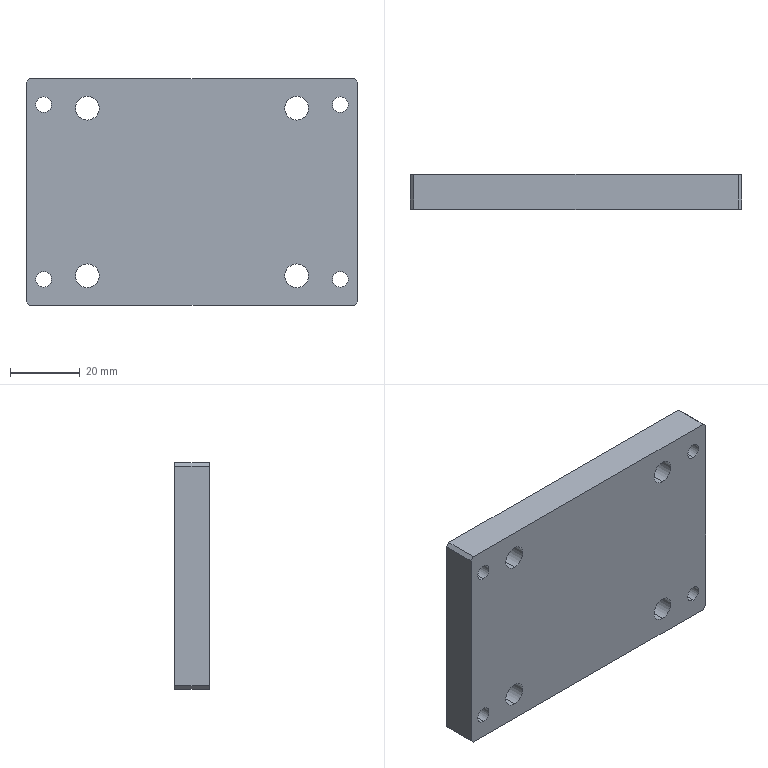Part | SolidWorks | features HoleWzd 2, Chamfer 1, Extrusion 1 | 1 solid | 38 faces | box 95 x 10 x 65 mm | volume 59009 mm3 | cylinder 24 | plane 14 | commonest cylinder face diameters 4.5 x8 6.8 x8 8 x8
STEP:
#1=CARTESIAN_POINT('',(30.,-5.,-27.4));
#2=VERTEX_POINT('',#1);
#3=CARTESIAN_POINT('',(30.,-5.,-20.6));
#4=VERTEX_POINT('',#3);
#5=CARTESIAN_POINT('',(30.,-5.,-24.));
#6=DIRECTION('',(0.,1.,0.));
#7=DIRECTION('',(0.,0.,1.));
#8=AXIS2_PLACEMENT_3D('',#5,#6,#7);
#9=CIRCLE('',#8,3.4);
#10=EDGE_CURVE('',#2,#4,#9,.T.);
#11=ORIENTED_EDGE('',*,*,#10,.F.);
#12=CARTESIAN_POINT('',(30.,5.,-27.4));
#13=VERTEX_POINT('',#12);
#14=CARTESIAN_POINT('',(30.,5.,-27.4));
#15=DIRECTION('',(0.,1.,0.));
#16=VECTOR('',#15,1000.);
#17=LINE('',#14,#16);
#18=EDGE_CURVE('',#2,#13,#17,.T.);
#19=ORIENTED_EDGE('',*,*,#18,.T.);
#20=CARTESIAN_POINT('',(30.,5.,-20.6));
#21=VERTEX_POINT('',#20);
#22=CARTESIAN_POINT('',(30.,5.,-24.));
#23=DIRECTION('',(0.,1.,0.));
#24=DIRECTION('',(0.,0.,1.));
#25=AXIS2_PLACEMENT_3D('',#22,#23,#24);
#26=CIRCLE('',#25,3.4);
#27=EDGE_CURVE('',#13,#21,#26,.T.);
#28=ORIENTED_EDGE('',*,*,#27,.T.);
#29=CARTESIAN_POINT('',(30.,5.,-20.6));
#30=DIRECTION('',(0.,1.,0.));
#31=VECTOR('',#30,1000.);
#32=LINE('',#29,#31);
#33=EDGE_CURVE('',#4,#21,#32,.T.);
#34=ORIENTED_EDGE('',*,*,#33,.F.);
#35=EDGE_LOOP('',(#11,#19,#28,#34));
#36=FACE_OUTER_BOUND('',#35,.T.);
#37=CARTESIAN_POINT('',(30.,5.,-24.));
#38=DIRECTION('',(0.,1.,0.));
#39=DIRECTION('',(0.,0.,1.));
#40=AXIS2_PLACEMENT_3D('',#37,#38,#39);
#41=CYLINDRICAL_SURFACE('',#40,3.4);
#42=ADVANCED_FACE('',(#36),#41,.F.);
#43=CARTESIAN_POINT('',(30.,-5.,20.6));
#44=VERTEX_POINT('',#43);
#45=CARTESIAN_POINT('',(30.,-5.,27.4));
#46=VERTEX_POINT('',#45);
#47=CARTESIAN_POINT('',(30.,-5.,24.));
#48=DIRECTION('',(0.,1.,0.));
#49=DIRECTION('',(0.,0.,1.));
#50=AXIS2_PLACEMENT_3D('',#47,#48,#49);
#51=CIRCLE('',#50,3.4);
#52=EDGE_CURVE('',#44,#46,#51,.T.);
#53=ORIENTED_EDGE('',*,*,#52,.F.);
#54=CARTESIAN_POINT('',(30.,5.,20.6));
#55=VERTEX_POINT('',#54);
#56=CARTESIAN_POINT('',(30.,5.,20.6));
#57=DIRECTION('',(0.,1.,0.));
#58=VECTOR('',#57,1000.);
#59=LINE('',#56,#58);
#60=EDGE_CURVE('',#44,#55,#59,.T.);
#61=ORIENTED_EDGE('',*,*,#60,.T.);
#62=CARTESIAN_POINT('',(30.,5.,27.4));
#63=VERTEX_POINT('',#62);
#64=CARTESIAN_POINT('',(30.,5.,24.));
#65=DIRECTION('',(0.,1.,0.));
#66=DIRECTION('',(0.,0.,1.));
#67=AXIS2_PLACEMENT_3D('',#64,#65,#66);
#68=CIRCLE('',#67,3.4);
#69=EDGE_CURVE('',#55,#63,#68,.T.);
#70=ORIENTED_EDGE('',*,*,#69,.T.);
#71=CARTESIAN_POINT('',(30.,5.,27.4));
#72=DIRECTION('',(0.,1.,0.));
#73=VECTOR('',#72,1000.);
#74=LINE('',#71,#73);
#75=EDGE_CURVE('',#46,#63,#74,.T.);
#76=ORIENTED_EDGE('',*,*,#75,.F.);
#77=EDGE_LOOP('',(#53,#61,#70,#76));
#78=FACE_OUTER_BOUND('',#77,.T.);
#79=CARTESIAN_POINT('',(30.,5.,24.));
#80=DIRECTION('',(0.,1.,0.));
#81=DIRECTION('',(0.,0.,1.));
#82=AXIS2_PLACEMENT_3D('',#79,#80,#81);
#83=CYLINDRICAL_SURFACE('',#82,3.4);
#84=ADVANCED_FACE('',(#78),#83,.F.);
#85=CARTESIAN_POINT('',(-30.,-5.,20.6));
#86=VERTEX_POINT('',#85);
#87=CARTESIAN_POINT('',(-30.,-5.,27.4));
#88=VERTEX_POINT('',#87);
#89=CARTESIAN_POINT('',(-30.,-5.,24.));
#90=DIRECTION('',(0.,1.,0.));
#91=DIRECTION('',(0.,0.,1.));
#92=AXIS2_PLACEMENT_3D('',#89,#90,#91);
#93=CIRCLE('',#92,3.4);
#94=EDGE_CURVE('',#86,#88,#93,.T.);
#95=ORIENTED_EDGE('',*,*,#94,.F.);
#96=CARTESIAN_POINT('',(-30.,5.,20.6));
#97=VERTEX_POINT('',#96);
#98=CARTESIAN_POINT('',(-30.,5.,20.6));
#99=DIRECTION('',(0.,1.,0.));
#100=VECTOR('',#99,1000.);
#101=LINE('',#98,#100);
#102=EDGE_CURVE('',#86,#97,#101,.T.);
#103=ORIENTED_EDGE('',*,*,#102,.T.);
#104=CARTESIAN_POINT('',(-30.,5.,27.4));
#105=VERTEX_POINT('',#104);
#106=CARTESIAN_POINT('',(-30.,5.,24.));
#107=DIRECTION('',(0.,1.,0.));
#108=DIRECTION('',(0.,0.,1.));
#109=AXIS2_PLACEMENT_3D('',#106,#107,#108);
#110=CIRCLE('',#109,3.4);
#111=EDGE_CURVE('',#97,#105,#110,.T.);
#112=ORIENTED_EDGE('',*,*,#111,.T.);
#113=CARTESIAN_POINT('',(-30.,5.,27.4));
#114=DIRECTION('',(0.,1.,0.));
#115=VECTOR('',#114,1000.);
#116=LINE('',#113,#115);
#117=EDGE_CURVE('',#88,#105,#116,.T.);
#118=ORIENTED_EDGE('',*,*,#117,.F.);
#119=EDGE_LOOP('',(#95,#103,#112,#118));
#120=FACE_OUTER_BOUND('',#119,.T.);
#121=CARTESIAN_POINT('',(-30.,5.,24.));
#122=DIRECTION('',(0.,1.,0.));
#123=DIRECTION('',(0.,0.,1.));
#124=AXIS2_PLACEMENT_3D('',#121,#122,#123);
#125=CYLINDRICAL_SURFACE('',#124,3.4);
#126=ADVANCED_FACE('',(#120),#125,.F.);
#127=CARTESIAN_POINT('',(-30.,-5.,-27.4));
#128=VERTEX_POINT('',#127);
#129=CARTESIAN_POINT('',(-30.,-5.,-20.6));
#130=VERTEX_POINT('',#129);
#131=CARTESIAN_POINT('',(-30.,-5.,-24.));
#132=DIRECTION('',(0.,1.,0.));
#133=DIRECTION('',(0.,0.,1.));
#134=AXIS2_PLACEMENT_3D('',#131,#132,#133);
#135=CIRCLE('',#134,3.4);
#136=EDGE_CURVE('',#128,#130,#135,.T.);
#137=ORIENTED_EDGE('',*,*,#136,.F.);
#138=CARTESIAN_POINT('',(-30.,5.,-27.4));
#139=VERTEX_POINT('',#138);
#140=CARTESIAN_POINT('',(-30.,5.,-27.4));
#141=DIRECTION('',(0.,1.,0.));
#142=VECTOR('',#141,1000.);
#143=LINE('',#140,#142);
#144=EDGE_CURVE('',#128,#139,#143,.T.);
#145=ORIENTED_EDGE('',*,*,#144,.T.);
#146=CARTESIAN_POINT('',(-30.,5.,-20.6));
#147=VERTEX_POINT('',#146);
#148=CARTESIAN_POINT('',(-30.,5.,-24.));
#149=DIRECTION('',(0.,1.,0.));
#150=DIRECTION('',(0.,0.,1.));
#151=AXIS2_PLACEMENT_3D('',#148,#149,#150);
#152=CIRCLE('',#151,3.4);
#153=EDGE_CURVE('',#139,#147,#152,.T.);
#154=ORIENTED_EDGE('',*,*,#153,.T.);
#155=CARTESIAN_POINT('',(-30.,5.,-20.6));
#156=DIRECTION('',(0.,1.,0.));
#157=VECTOR('',#156,1000.);
#158=LINE('',#155,#157);
#159=EDGE_CURVE('',#130,#147,#158,.T.);
#160=ORIENTED_EDGE('',*,*,#159,.F.);
#161=EDGE_LOOP('',(#137,#145,#154,#160));
#162=FACE_OUTER_BOUND('',#161,.T.);
#163=CARTESIAN_POINT('',(-30.,5.,-24.));
#164=DIRECTION('',(0.,1.,0.));
#165=DIRECTION('',(0.,0.,1.));
#166=AXIS2_PLACEMENT_3D('',#163,#164,#165);
#167=CYLINDRICAL_SURFACE('',#166,3.4);
#168=ADVANCED_FACE('',(#162),#167,.F.);
#169=CARTESIAN_POINT('',(-42.5,0.4,-29.));
#170=VERTEX_POINT('',#169);
#171=CARTESIAN_POINT('',(-42.5,0.4,-21.));
#172=VERTEX_POINT('',#171);
#173=CARTESIAN_POINT('',(-42.5,0.4,-25.));
#174=DIRECTION('',(0.,1.,0.));
#175=DIRECTION('',(0.,0.,1.));
#176=AXIS2_PLACEMENT_3D('',#173,#174,#175);
#177=CIRCLE('',#176,4.);
#178=EDGE_CURVE('',#170,#172,#177,.T.);
#179=ORIENTED_EDGE('',*,*,#178,.F.);
#180=CARTESIAN_POINT('',(-42.5,5.,-29.));
#181=VERTEX_POINT('',#180);
#182=CARTESIAN_POINT('',(-42.5,5.,-29.));
#183=DIRECTION('',(0.,1.,0.));
#184=VECTOR('',#183,1000.);
#185=LINE('',#182,#184);
#186=EDGE_CURVE('',#170,#181,#185,.T.);
#187=ORIENTED_EDGE('',*,*,#186,.T.);
#188=CARTESIAN_POINT('',(-42.5,5.,-21.));
#189=VERTEX_POINT('',#188);
#190=CARTESIAN_POINT('',(-42.5,5.,-25.));
#191=DIRECTION('',(0.,1.,0.));
#192=DIRECTION('',(0.,0.,1.));
#193=AXIS2_PLACEMENT_3D('',#190,#191,#192);
#194=CIRCLE('',#193,4.);
#195=EDGE_CURVE('',#181,#189,#194,.T.);
#196=ORIENTED_EDGE('',*,*,#195,.T.);
#197=CARTESIAN_POINT('',(-42.5,5.,-21.));
#198=DIRECTION('',(0.,1.,0.));
#199=VECTOR('',#198,1000.);
#200=LINE('',#197,#199);
#201=EDGE_CURVE('',#172,#189,#200,.T.);
#202=ORIENTED_EDGE('',*,*,#201,.F.);
#203=EDGE_LOOP('',(#179,#187,#196,#202));
#204=FACE_OUTER_BOUND('',#203,.T.);
#205=CARTESIAN_POINT('',(-42.5,5.,-25.));
#206=DIRECTION('',(0.,1.,0.));
#207=DIRECTION('',(0.,0.,1.));
#208=AXIS2_PLACEMENT_3D('',#205,#206,#207);
#209=CYLINDRICAL_SURFACE('',#208,4.);
#210=ADVANCED_FACE('',(#204),#209,.F.);
#211=CARTESIAN_POINT('',(-42.5,-5.,-27.25));
#212=VERTEX_POINT('',#211);
#213=CARTESIAN_POINT('',(-42.5,-5.,-22.75));
#214=VERTEX_POINT('',#213);
#215=CARTESIAN_POINT('',(-42.5,-5.,-25.));
#216=DIRECTION('',(0.,1.,0.));
#217=DIRECTION('',(0.,0.,1.));
#218=AXIS2_PLACEMENT_3D('',#215,#216,#217);
#219=CIRCLE('',#218,2.25);
#220=EDGE_CURVE('',#212,#214,#219,.T.);
#221=ORIENTED_EDGE('',*,*,#220,.F.);
#222=CARTESIAN_POINT('',(-42.5,0.4,-27.25));
#223=VERTEX_POINT('',#222);
#224=CARTESIAN_POINT('',(-42.5,5.,-27.25));
#225=DIRECTION('',(0.,1.,0.));
#226=VECTOR('',#225,1000.);
#227=LINE('',#224,#226);
#228=EDGE_CURVE('',#212,#223,#227,.T.);
#229=ORIENTED_EDGE('',*,*,#228,.T.);
#230=CARTESIAN_POINT('',(-42.5,0.4,-22.75));
#231=VERTEX_POINT('',#230);
#232=CARTESIAN_POINT('',(-42.5,0.4,-25.));
#233=DIRECTION('',(0.,1.,0.));
#234=DIRECTION('',(0.,0.,1.));
#235=AXIS2_PLACEMENT_3D('',#232,#233,#234);
#236=CIRCLE('',#235,2.25);
#237=EDGE_CURVE('',#223,#231,#236,.T.);
#238=ORIENTED_EDGE('',*,*,#237,.T.);
#239=CARTESIAN_POINT('',(-42.5,5.,-22.75));
#240=DIRECTION('',(0.,1.,0.));
#241=VECTOR('',#240,1000.);
#242=LINE('',#239,#241);
#243=EDGE_CURVE('',#214,#231,#242,.T.);
#244=ORIENTED_EDGE('',*,*,#243,.F.);
#245=EDGE_LOOP('',(#221,#229,#238,#244));
#246=FACE_OUTER_BOUND('',#245,.T.);
#247=CARTESIAN_POINT('',(-42.5,5.,-25.));
#248=DIRECTION('',(0.,1.,0.));
#249=DIRECTION('',(0.,0.,1.));
#250=AXIS2_PLACEMENT_3D('',#247,#248,#249);
#251=CYLINDRICAL_SURFACE('',#250,2.25);
#252=ADVANCED_FACE('',(#246),#251,.F.);
#253=CARTESIAN_POINT('',(-42.5,0.4,21.));
#254=VERTEX_POINT('',#253);
#255=CARTESIAN_POINT('',(-42.5,0.4,29.));
#256=VERTEX_POINT('',#255);
#257=CARTESIAN_POINT('',(-42.5,0.4,25.));
#258=DIRECTION('',(0.,1.,0.));
#259=DIRECTION('',(0.,0.,1.));
#260=AXIS2_PLACEMENT_3D('',#257,#258,#259);
#261=CIRCLE('',#260,4.);
#262=EDGE_CURVE('',#254,#256,#261,.T.);
#263=ORIENTED_EDGE('',*,*,#262,.F.);
#264=CARTESIAN_POINT('',(-42.5,5.,21.));
#265=VERTEX_POINT('',#264);
#266=CARTESIAN_POINT('',(-42.5,5.,21.));
#267=DIRECTION('',(0.,1.,0.));
#268=VECTOR('',#267,1000.);
#269=LINE('',#266,#268);
#270=EDGE_CURVE('',#254,#265,#269,.T.);
#271=ORIENTED_EDGE('',*,*,#270,.T.);
#272=CARTESIAN_POINT('',(-42.5,5.,29.));
#273=VERTEX_POINT('',#272);
#274=CARTESIAN_POINT('',(-42.5,5.,25.));
#275=DIRECTION('',(0.,1.,0.));
#276=DIRECTION('',(0.,0.,1.));
#277=AXIS2_PLACEMENT_3D('',#274,#275,#276);
#278=CIRCLE('',#277,4.);
#279=EDGE_CURVE('',#265,#273,#278,.T.);
#280=ORIENTED_EDGE('',*,*,#279,.T.);
#281=CARTESIAN_POINT('',(-42.5,5.,29.));
#282=DIRECTION('',(0.,1.,0.));
#283=VECTOR('',#282,1000.);
#284=LINE('',#281,#283);
#285=EDGE_CURVE('',#256,#273,#284,.T.);
#286=ORIENTED_EDGE('',*,*,#285,.F.);
#287=EDGE_LOOP('',(#263,#271,#280,#286));
#288=FACE_OUTER_BOUND('',#287,.T.);
#289=CARTESIAN_POINT('',(-42.5,5.,25.));
#290=DIRECTION('',(0.,1.,0.));
#291=DIRECTION('',(0.,0.,1.));
#292=AXIS2_PLACEMENT_3D('',#289,#290,#291);
#293=CYLINDRICAL_SURFACE('',#292,4.);
#294=ADVANCED_FACE('',(#288),#293,.F.);
#295=CARTESIAN_POINT('',(-42.5,-5.,22.75));
#296=VERTEX_POINT('',#295);
#297=CARTESIAN_POINT('',(-42.5,-5.,27.25));
#298=VERTEX_POINT('',#297);
#299=CARTESIAN_POINT('',(-42.5,-5.,25.));
#300=DIRECTION('',(0.,1.,0.));
#301=DIRECTION('',(0.,0.,1.));
#302=AXIS2_PLACEMENT_3D('',#299,#300,#301);
#303=CIRCLE('',#302,2.25);
#304=EDGE_CURVE('',#296,#298,#303,.T.);
#305=ORIENTED_EDGE('',*,*,#304,.F.);
#306=CARTESIAN_POINT('',(-42.5,0.4,22.75));
#307=VERTEX_POINT('',#306);
#308=CARTESIAN_POINT('',(-42.5,5.,22.75));
#309=DIRECTION('',(0.,1.,0.));
#310=VECTOR('',#309,1000.);
#311=LINE('',#308,#310);
#312=EDGE_CURVE('',#296,#307,#311,.T.);
#313=ORIENTED_EDGE('',*,*,#312,.T.);
#314=CARTESIAN_POINT('',(-42.5,0.4,27.25));
#315=VERTEX_POINT('',#314);
#316=CARTESIAN_POINT('',(-42.5,0.4,25.));
#317=DIRECTION('',(0.,1.,0.));
#318=DIRECTION('',(0.,0.,1.));
#319=AXIS2_PLACEMENT_3D('',#316,#317,#318);
#320=CIRCLE('',#319,2.25);
#321=EDGE_CURVE('',#307,#315,#320,.T.);
#322=ORIENTED_EDGE('',*,*,#321,.T.);
#323=CARTESIAN_POINT('',(-42.5,5.,27.25));
#324=DIRECTION('',(0.,1.,0.));
#325=VECTOR('',#324,1000.);
#326=LINE('',#323,#325);
#327=EDGE_CURVE('',#298,#315,#326,.T.);
#328=ORIENTED_EDGE('',*,*,#327,.F.);
#329=EDGE_LOOP('',(#305,#313,#322,#328));
#330=FACE_OUTER_BOUND('',#329,.T.);
#331=CARTESIAN_POINT('',(-42.5,5.,25.));
#332=DIRECTION('',(0.,1.,0.));
#333=DIRECTION('',(0.,0.,1.));
#334=AXIS2_PLACEMENT_3D('',#331,#332,#333);
#335=CYLINDRICAL_SURFACE('',#334,2.25);
#336=ADVANCED_FACE('',(#330),#335,.F.);
#337=CARTESIAN_POINT('',(42.5,0.4,21.));
#338=VERTEX_POINT('',#337);
#339=CARTESIAN_POINT('',(42.5,0.4,29.));
#340=VERTEX_POINT('',#339);
#341=CARTESIAN_POINT('',(42.5,0.4,25.));
#342=DIRECTION('',(0.,1.,0.));
#343=DIRECTION('',(0.,0.,1.));
#344=AXIS2_PLACEMENT_3D('',#341,#342,#343);
#345=CIRCLE('',#344,4.);
#346=EDGE_CURVE('',#338,#340,#345,.T.);
#347=ORIENTED_EDGE('',*,*,#346,.F.);
#348=CARTESIAN_POINT('',(42.5,5.,21.));
#349=VERTEX_POINT('',#348);
#350=CARTESIAN_POINT('',(42.5,5.,21.));
#351=DIRECTION('',(0.,1.,0.));
#352=VECTOR('',#351,1000.);
#353=LINE('',#350,#352);
#354=EDGE_CURVE('',#338,#349,#353,.T.);
#355=ORIENTED_EDGE('',*,*,#354,.T.);
#356=CARTESIAN_POINT('',(42.5,5.,29.));
#357=VERTEX_POINT('',#356);
#358=CARTESIAN_POINT('',(42.5,5.,25.));
#359=DIRECTION('',(0.,1.,0.));
#360=DIRECTION('',(0.,0.,1.));
#361=AXIS2_PLACEMENT_3D('',#358,#359,#360);
#362=CIRCLE('',#361,4.);
#363=EDGE_CURVE('',#349,#357,#362,.T.);
#364=ORIENTED_EDGE('',*,*,#363,.T.);
#365=CARTESIAN_POINT('',(42.5,5.,29.));
#366=DIRECTION('',(0.,1.,0.));
#367=VECTOR('',#366,1000.);
#368=LINE('',#365,#367);
#369=EDGE_CURVE('',#340,#357,#368,.T.);
#370=ORIENTED_EDGE('',*,*,#369,.F.);
#371=EDGE_LOOP('',(#347,#355,#364,#370));
#372=FACE_OUTER_BOUND('',#371,.T.);
#373=CARTESIAN_POINT('',(42.5,5.,25.));
#374=DIRECTION('',(0.,1.,0.));
#375=DIRECTION('',(0.,0.,1.));
#376=AXIS2_PLACEMENT_3D('',#373,#374,#375);
#377=CYLINDRICAL_SURFACE('',#376,4.);
#378=ADVANCED_FACE('',(#372),#377,.F.);
#379=CARTESIAN_POINT('',(42.5,-5.,22.75));
#380=VERTEX_POINT('',#379);
#381=CARTESIAN_POINT('',(42.5,-5.,27.25));
#382=VERTEX_POINT('',#381);
#383=CARTESIAN_POINT('',(42.5,-5.,25.));
#384=DIRECTION('',(0.,1.,0.));
#385=DIRECTION('',(0.,0.,1.));
#386=AXIS2_PLACEMENT_3D('',#383,#384,#385);
#387=CIRCLE('',#386,2.25);
#388=EDGE_CURVE('',#380,#382,#387,.T.);
#389=ORIENTED_EDGE('',*,*,#388,.F.);
#390=CARTESIAN_POINT('',(42.5,0.4,22.75));
#391=VERTEX_POINT('',#390);
#392=CARTESIAN_POINT('',(42.5,5.,22.75));
#393=DIRECTION('',(0.,1.,0.));
#394=VECTOR('',#393,1000.);
#395=LINE('',#392,#394);
#396=EDGE_CURVE('',#380,#391,#395,.T.);
#397=ORIENTED_EDGE('',*,*,#396,.T.);
#398=CARTESIAN_POINT('',(42.5,0.4,27.25));
#399=VERTEX_POINT('',#398);
#400=CARTESIAN_POINT('',(42.5,0.4,25.));
#401=DIRECTION('',(0.,1.,0.));
#402=DIRECTION('',(0.,0.,1.));
#403=AXIS2_PLACEMENT_3D('',#400,#401,#402);
#404=CIRCLE('',#403,2.25);
#405=EDGE_CURVE('',#391,#399,#404,.T.);
#406=ORIENTED_EDGE('',*,*,#405,.T.);
#407=CARTESIAN_POINT('',(42.5,5.,27.25));
#408=DIRECTION('',(0.,1.,0.));
#409=VECTOR('',#408,1000.);
#410=LINE('',#407,#409);
#411=EDGE_CURVE('',#382,#399,#410,.T.);
#412=ORIENTED_EDGE('',*,*,#411,.F.);
#413=EDGE_LOOP('',(#389,#397,#406,#412));
#414=FACE_OUTER_BOUND('',#413,.T.);
#415=CARTESIAN_POINT('',(42.5,5.,25.));
#416=DIRECTION('',(0.,1.,0.));
#417=DIRECTION('',(0.,0.,1.));
#418=AXIS2_PLACEMENT_3D('',#415,#416,#417);
#419=CYLINDRICAL_SURFACE('',#418,2.25);
#420=ADVANCED_FACE('',(#414),#419,.F.);
#421=CARTESIAN_POINT('',(42.5,0.4,-29.));
#422=VERTEX_POINT('',#421);
#423=CARTESIAN_POINT('',(42.5,0.4,-21.));
#424=VERTEX_POINT('',#423);
#425=CARTESIAN_POINT('',(42.5,0.4,-25.));
#426=DIRECTION('',(0.,1.,0.));
#427=DIRECTION('',(0.,0.,1.));
#428=AXIS2_PLACEMENT_3D('',#425,#426,#427);
#429=CIRCLE('',#428,4.);
#430=EDGE_CURVE('',#422,#424,#429,.T.);
#431=ORIENTED_EDGE('',*,*,#430,.F.);
#432=CARTESIAN_POINT('',(42.5,5.,-29.));
#433=VERTEX_POINT('',#432);
#434=CARTESIAN_POINT('',(42.5,5.,-29.));
#435=DIRECTION('',(0.,1.,0.));
#436=VECTOR('',#435,1000.);
#437=LINE('',#434,#436);
#438=EDGE_CURVE('',#422,#433,#437,.T.);
#439=ORIENTED_EDGE('',*,*,#438,.T.);
#440=CARTESIAN_POINT('',(42.5,5.,-21.));
#441=VERTEX_POINT('',#440);
#442=CARTESIAN_POINT('',(42.5,5.,-25.));
#443=DIRECTION('',(0.,1.,0.));
#444=DIRECTION('',(0.,0.,1.));
#445=AXIS2_PLACEMENT_3D('',#442,#443,#444);
#446=CIRCLE('',#445,4.);
#447=EDGE_CURVE('',#433,#441,#446,.T.);
#448=ORIENTED_EDGE('',*,*,#447,.T.);
#449=CARTESIAN_POINT('',(42.5,5.,-21.));
#450=DIRECTION('',(0.,1.,0.));
#451=VECTOR('',#450,1000.);
#452=LINE('',#449,#451);
#453=EDGE_CURVE('',#424,#441,#452,.T.);
#454=ORIENTED_EDGE('',*,*,#453,.F.);
#455=EDGE_LOOP('',(#431,#439,#448,#454));
#456=FACE_OUTER_BOUND('',#455,.T.);
#457=CARTESIAN_POINT('',(42.5,5.,-25.));
#458=DIRECTION('',(0.,1.,0.));
#459=DIRECTION('',(0.,0.,1.));
#460=AXIS2_PLACEMENT_3D('',#457,#458,#459);
#461=CYLINDRICAL_SURFACE('',#460,4.);
#462=ADVANCED_FACE('',(#456),#461,.F.);
#463=CARTESIAN_POINT('',(42.5,-5.,-27.25));
#464=VERTEX_POINT('',#463);
#465=CARTESIAN_POINT('',(42.5,-5.,-22.75));
#466=VERTEX_POINT('',#465);
#467=CARTESIAN_POINT('',(42.5,-5.,-25.));
#468=DIRECTION('',(0.,1.,0.));
#469=DIRECTION('',(0.,0.,1.));
#470=AXIS2_PLACEMENT_3D('',#467,#468,#469);
#471=CIRCLE('',#470,2.25);
#472=EDGE_CURVE('',#464,#466,#471,.T.);
#473=ORIENTED_EDGE('',*,*,#472,.F.);
#474=CARTESIAN_POINT('',(42.5,0.4,-27.25));
#475=VERTEX_POINT('',#474);
#476=CARTESIAN_POINT('',(42.5,5.,-27.25));
#477=DIRECTION('',(0.,1.,0.));
#478=VECTOR('',#477,1000.);
#479=LINE('',#476,#478);
#480=EDGE_CURVE('',#464,#475,#479,.T.);
#481=ORIENTED_EDGE('',*,*,#480,.T.);
#482=CARTESIAN_POINT('',(42.5,0.4,-22.75));
#483=VERTEX_POINT('',#482);
#484=CARTESIAN_POINT('',(42.5,0.4,-25.));
#485=DIRECTION('',(0.,1.,0.));
#486=DIRECTION('',(0.,0.,1.));
#487=AXIS2_PLACEMENT_3D('',#484,#485,#486);
#488=CIRCLE('',#487,2.25);
#489=EDGE_CURVE('',#475,#483,#488,.T.);
#490=ORIENTED_EDGE('',*,*,#489,.T.);
#491=CARTESIAN_POINT('',(42.5,5.,-22.75));
#492=DIRECTION('',(0.,1.,0.));
#493=VECTOR('',#492,1000.);
#494=LINE('',#491,#493);
#495=EDGE_CURVE('',#466,#483,#494,.T.);
#496=ORIENTED_EDGE('',*,*,#495,.F.);
#497=EDGE_LOOP('',(#473,#481,#490,#496));
#498=FACE_OUTER_BOUND('',#497,.T.);
#499=CARTESIAN_POINT('',(42.5,5.,-25.));
#500=DIRECTION('',(0.,1.,0.));
#501=DIRECTION('',(0.,0.,1.));
#502=AXIS2_PLACEMENT_3D('',#499,#500,#501);
#503=CYLINDRICAL_SURFACE('',#502,2.25);
#504=ADVANCED_FACE('',(#498),#503,.F.);
#505=CARTESIAN_POINT('',(30.,-5.,-24.));
#506=DIRECTION('',(0.,1.,0.));
#507=DIRECTION('',(0.,0.,1.));
#508=AXIS2_PLACEMENT_3D('',#505,#506,#507);
#509=CIRCLE('',#508,3.4);
#510=EDGE_CURVE('',#4,#2,#509,.T.);
#511=ORIENTED_EDGE('',*,*,#510,.T.);
#512=ORIENTED_EDGE('',*,*,#10,.T.);
#513=EDGE_LOOP('',(#511,#512));
#514=FACE_BOUND('',#513,.T.);
#515=CARTESIAN_POINT('',(30.,-5.,24.));
#516=DIRECTION('',(0.,1.,0.));
#517=DIRECTION('',(0.,0.,1.));
#518=AXIS2_PLACEMENT_3D('',#515,#516,#517);
#519=CIRCLE('',#518,3.4);
#520=EDGE_CURVE('',#46,#44,#519,.T.);
#521=ORIENTED_EDGE('',*,*,#520,.T.);
#522=ORIENTED_EDGE('',*,*,#52,.T.);
#523=EDGE_LOOP('',(#521,#522));
#524=FACE_BOUND('',#523,.T.);
#525=CARTESIAN_POINT('',(-30.,-5.,24.));
#526=DIRECTION('',(0.,1.,0.));
#527=DIRECTION('',(0.,0.,1.));
#528=AXIS2_PLACEMENT_3D('',#525,#526,#527);
#529=CIRCLE('',#528,3.4);
#530=EDGE_CURVE('',#88,#86,#529,.T.);
#531=ORIENTED_EDGE('',*,*,#530,.T.);
#532=ORIENTED_EDGE('',*,*,#94,.T.);
#533=EDGE_LOOP('',(#531,#532));
#534=FACE_BOUND('',#533,.T.);
#535=CARTESIAN_POINT('',(46.5,-5.,-32.5));
#536=VERTEX_POINT('',#535);
#537=CARTESIAN_POINT('',(-46.5,-5.,-32.5));
#538=VERTEX_POINT('',#537);
#539=CARTESIAN_POINT('',(-47.5,-5.,-32.5));
#540=DIRECTION('',(-1.,0.,0.));
#541=VECTOR('',#540,1000.);
#542=LINE('',#539,#541);
#543=EDGE_CURVE('',#536,#538,#542,.T.);
#544=ORIENTED_EDGE('',*,*,#543,.F.);
#545=CARTESIAN_POINT('',(47.5,-5.,-31.5));
#546=VERTEX_POINT('',#545);
#547=CARTESIAN_POINT('',(39.5,-5.,-39.5));
#548=DIRECTION('',(0.7071,0.,0.7071));
#549=VECTOR('',#548,1000.);
#550=LINE('',#547,#549);
#551=EDGE_CURVE('',#536,#546,#550,.T.);
#552=ORIENTED_EDGE('',*,*,#551,.T.);
#553=CARTESIAN_POINT('',(47.5,-5.,31.5));
#554=VERTEX_POINT('',#553);
#555=CARTESIAN_POINT('',(47.5,-5.,32.5));
#556=DIRECTION('',(0.,0.,-1.));
#557=VECTOR('',#556,1000.);
#558=LINE('',#555,#557);
#559=EDGE_CURVE('',#554,#546,#558,.T.);
#560=ORIENTED_EDGE('',*,*,#559,.F.);
#561=CARTESIAN_POINT('',(46.5,-5.,32.5));
#562=VERTEX_POINT('',#561);
#563=CARTESIAN_POINT('',(39.5,-5.,39.5));
#564=DIRECTION('',(-0.7071,0.,0.7071));
#565=VECTOR('',#564,1000.);
#566=LINE('',#563,#565);
#567=EDGE_CURVE('',#554,#562,#566,.T.);
#568=ORIENTED_EDGE('',*,*,#567,.T.);
#569=CARTESIAN_POINT('',(-46.5,-5.,32.5));
#570=VERTEX_POINT('',#569);
#571=CARTESIAN_POINT('',(-47.5,-5.,32.5));
#572=DIRECTION('',(1.,0.,0.));
#573=VECTOR('',#572,1000.);
#574=LINE('',#571,#573);
#575=EDGE_CURVE('',#570,#562,#574,.T.);
#576=ORIENTED_EDGE('',*,*,#575,.F.);
#577=CARTESIAN_POINT('',(-47.5,-5.,31.5));
#578=VERTEX_POINT('',#577);
#579=CARTESIAN_POINT('',(-39.5,-5.,39.5));
#580=DIRECTION('',(-0.7071,0.,-0.7071));
#581=VECTOR('',#580,1000.);
#582=LINE('',#579,#581);
#583=EDGE_CURVE('',#570,#578,#582,.T.);
#584=ORIENTED_EDGE('',*,*,#583,.T.);
#585=CARTESIAN_POINT('',(-47.5,-5.,-31.5));
#586=VERTEX_POINT('',#585);
#587=CARTESIAN_POINT('',(-47.5,-5.,32.5));
#588=DIRECTION('',(0.,0.,1.));
#589=VECTOR('',#588,1000.);
#590=LINE('',#587,#589);
#591=EDGE_CURVE('',#586,#578,#590,.T.);
#592=ORIENTED_EDGE('',*,*,#591,.F.);
#593=CARTESIAN_POINT('',(-39.5,-5.,-39.5));
#594=DIRECTION('',(0.7071,0.,-0.7071));
#595=VECTOR('',#594,1000.);
#596=LINE('',#593,#595);
#597=EDGE_CURVE('',#586,#538,#596,.T.);
#598=ORIENTED_EDGE('',*,*,#597,.T.);
#599=EDGE_LOOP('',(#544,#552,#560,#568,#576,#584,#592,#598));
#600=FACE_OUTER_BOUND('',#599,.T.);
#601=CARTESIAN_POINT('',(42.5,-5.,-25.));
#602=DIRECTION('',(0.,1.,0.));
#603=DIRECTION('',(0.,0.,1.));
#604=AXIS2_PLACEMENT_3D('',#601,#602,#603);
#605=CIRCLE('',#604,2.25);
#606=EDGE_CURVE('',#466,#464,#605,.T.);
#607=ORIENTED_EDGE('',*,*,#606,.T.);
#608=ORIENTED_EDGE('',*,*,#472,.T.);
#609=EDGE_LOOP('',(#607,#608));
#610=FACE_BOUND('',#609,.T.);
#611=CARTESIAN_POINT('',(42.5,-5.,25.));
#612=DIRECTION('',(0.,1.,0.));
#613=DIRECTION('',(0.,0.,1.));
#614=AXIS2_PLACEMENT_3D('',#611,#612,#613);
#615=CIRCLE('',#614,2.25);
#616=EDGE_CURVE('',#382,#380,#615,.T.);
#617=ORIENTED_EDGE('',*,*,#616,.T.);
#618=ORIENTED_EDGE('',*,*,#388,.T.);
#619=EDGE_LOOP('',(#617,#618));
#620=FACE_BOUND('',#619,.T.);
#621=CARTESIAN_POINT('',(-42.5,-5.,25.));
#622=DIRECTION('',(0.,1.,0.));
#623=DIRECTION('',(0.,0.,1.));
#624=AXIS2_PLACEMENT_3D('',#621,#622,#623);
#625=CIRCLE('',#624,2.25);
#626=EDGE_CURVE('',#298,#296,#625,.T.);
#627=ORIENTED_EDGE('',*,*,#626,.T.);
#628=ORIENTED_EDGE('',*,*,#304,.T.);
#629=EDGE_LOOP('',(#627,#628));
#630=FACE_BOUND('',#629,.T.);
#631=CARTESIAN_POINT('',(-42.5,-5.,-25.));
#632=DIRECTION('',(0.,1.,0.));
#633=DIRECTION('',(0.,0.,1.));
#634=AXIS2_PLACEMENT_3D('',#631,#632,#633);
#635=CIRCLE('',#634,2.25);
#636=EDGE_CURVE('',#214,#212,#635,.T.);
#637=ORIENTED_EDGE('',*,*,#636,.T.);
#638=ORIENTED_EDGE('',*,*,#220,.T.);
#639=EDGE_LOOP('',(#637,#638));
#640=FACE_BOUND('',#639,.T.);
#641=CARTESIAN_POINT('',(-30.,-5.,-24.));
#642=DIRECTION('',(0.,1.,0.));
#643=DIRECTION('',(0.,0.,1.));
#644=AXIS2_PLACEMENT_3D('',#641,#642,#643);
#645=CIRCLE('',#644,3.4);
#646=EDGE_CURVE('',#130,#128,#645,.T.);
#647=ORIENTED_EDGE('',*,*,#646,.T.);
#648=ORIENTED_EDGE('',*,*,#136,.T.);
#649=EDGE_LOOP('',(#647,#648));
#650=FACE_BOUND('',#649,.T.);
#651=CARTESIAN_POINT('',(0.,-5.,0.));
#652=DIRECTION('',(0.,-1.,0.));
#653=DIRECTION('',(0.,0.,-1.));
#654=AXIS2_PLACEMENT_3D('',#651,#652,#653);
#655=PLANE('',#654);
#656=ADVANCED_FACE('',(#514,#524,#534,#600,#610,#620,#630,#640,#650),#655,.T.);
#657=ORIENTED_EDGE('',*,*,#559,.T.);
#658=CARTESIAN_POINT('',(47.5,5.,-31.5));
#659=VERTEX_POINT('',#658);
#660=CARTESIAN_POINT('',(47.5,5.,-31.5));
#661=DIRECTION('',(0.,1.,0.));
#662=VECTOR('',#661,1000.);
#663=LINE('',#660,#662);
#664=EDGE_CURVE('',#546,#659,#663,.T.);
#665=ORIENTED_EDGE('',*,*,#664,.T.);
#666=CARTESIAN_POINT('',(47.5,5.,31.5));
#667=VERTEX_POINT('',#666);
#668=CARTESIAN_POINT('',(47.5,5.,32.5));
#669=DIRECTION('',(0.,0.,-1.));
#670=VECTOR('',#669,1000.);
#671=LINE('',#668,#670);
#672=EDGE_CURVE('',#667,#659,#671,.T.);
#673=ORIENTED_EDGE('',*,*,#672,.F.);
#674=CARTESIAN_POINT('',(47.5,5.,31.5));
#675=DIRECTION('',(0.,-1.,0.));
#676=VECTOR('',#675,1000.);
#677=LINE('',#674,#676);
#678=EDGE_CURVE('',#667,#554,#677,.T.);
#679=ORIENTED_EDGE('',*,*,#678,.T.);
#680=EDGE_LOOP('',(#657,#665,#673,#679));
#681=FACE_OUTER_BOUND('',#680,.T.);
#682=CARTESIAN_POINT('',(47.5,5.,32.5));
#683=DIRECTION('',(-1.,0.,0.));
#684=DIRECTION('',(0.,0.,1.));
#685=AXIS2_PLACEMENT_3D('',#682,#683,#684);
#686=PLANE('',#685);
#687=ADVANCED_FACE('',(#681),#686,.F.);
#688=CARTESIAN_POINT('',(46.5,5.,-32.5));
#689=VERTEX_POINT('',#688);
#690=CARTESIAN_POINT('',(-46.5,5.,-32.5));
#691=VERTEX_POINT('',#690);
#692=CARTESIAN_POINT('',(-47.5,5.,-32.5));
#693=DIRECTION('',(-1.,0.,0.));
#694=VECTOR('',#693,1000.);
#695=LINE('',#692,#694);
#696=EDGE_CURVE('',#689,#691,#695,.T.);
#697=ORIENTED_EDGE('',*,*,#696,.F.);
#698=CARTESIAN_POINT('',(46.5,5.,-32.5));
#699=DIRECTION('',(0.,-1.,0.));
#700=VECTOR('',#699,1000.);
#701=LINE('',#698,#700);
#702=EDGE_CURVE('',#689,#536,#701,.T.);
#703=ORIENTED_EDGE('',*,*,#702,.T.);
#704=ORIENTED_EDGE('',*,*,#543,.T.);
#705=CARTESIAN_POINT('',(-46.5,5.,-32.5));
#706=DIRECTION('',(0.,1.,0.));
#707=VECTOR('',#706,1000.);
#708=LINE('',#705,#707);
#709=EDGE_CURVE('',#538,#691,#708,.T.);
#710=ORIENTED_EDGE('',*,*,#709,.T.);
#711=EDGE_LOOP('',(#697,#703,#704,#710));
#712=FACE_OUTER_BOUND('',#711,.T.);
#713=CARTESIAN_POINT('',(-47.5,5.,-32.5));
#714=DIRECTION('',(0.,0.,1.));
#715=DIRECTION('',(1.,0.,0.));
#716=AXIS2_PLACEMENT_3D('',#713,#714,#715);
#717=PLANE('',#716);
#718=ADVANCED_FACE('',(#712),#717,.F.);
#719=ORIENTED_EDGE('',*,*,#591,.T.);
#720=CARTESIAN_POINT('',(-47.5,5.,31.5));
#721=VERTEX_POINT('',#720);
#722=CARTESIAN_POINT('',(-47.5,5.,31.5));
#723=DIRECTION('',(0.,1.,0.));
#724=VECTOR('',#723,1000.);
#725=LINE('',#722,#724);
#726=EDGE_CURVE('',#578,#721,#725,.T.);
#727=ORIENTED_EDGE('',*,*,#726,.T.);
#728=CARTESIAN_POINT('',(-47.5,5.,-31.5));
#729=VERTEX_POINT('',#728);
#730=CARTESIAN_POINT('',(-47.5,5.,32.5));
#731=DIRECTION('',(0.,0.,1.));
#732=VECTOR('',#731,1000.);
#733=LINE('',#730,#732);
#734=EDGE_CURVE('',#729,#721,#733,.T.);
#735=ORIENTED_EDGE('',*,*,#734,.F.);
#736=CARTESIAN_POINT('',(-47.5,5.,-31.5));
#737=DIRECTION('',(0.,-1.,0.));
#738=VECTOR('',#737,1000.);
#739=LINE('',#736,#738);
#740=EDGE_CURVE('',#729,#586,#739,.T.);
#741=ORIENTED_EDGE('',*,*,#740,.T.);
#742=EDGE_LOOP('',(#719,#727,#735,#741));
#743=FACE_OUTER_BOUND('',#742,.T.);
#744=CARTESIAN_POINT('',(-47.5,5.,32.5));
#745=DIRECTION('',(1.,0.,0.));
#746=DIRECTION('',(0.,0.,-1.));
#747=AXIS2_PLACEMENT_3D('',#744,#745,#746);
#748=PLANE('',#747);
#749=ADVANCED_FACE('',(#743),#748,.F.);
#750=ORIENTED_EDGE('',*,*,#575,.T.);
#751=CARTESIAN_POINT('',(46.5,5.,32.5));
#752=VERTEX_POINT('',#751);
#753=CARTESIAN_POINT('',(46.5,5.,32.5));
#754=DIRECTION('',(0.,1.,0.));
#755=VECTOR('',#754,1000.);
#756=LINE('',#753,#755);
#757=EDGE_CURVE('',#562,#752,#756,.T.);
#758=ORIENTED_EDGE('',*,*,#757,.T.);
#759=CARTESIAN_POINT('',(-46.5,5.,32.5));
#760=VERTEX_POINT('',#759);
#761=CARTESIAN_POINT('',(-47.5,5.,32.5));
#762=DIRECTION('',(1.,0.,0.));
#763=VECTOR('',#762,1000.);
#764=LINE('',#761,#763);
#765=EDGE_CURVE('',#760,#752,#764,.T.);
#766=ORIENTED_EDGE('',*,*,#765,.F.);
#767=CARTESIAN_POINT('',(-46.5,5.,32.5));
#768=DIRECTION('',(0.,-1.,0.));
#769=VECTOR('',#768,1000.);
#770=LINE('',#767,#769);
#771=EDGE_CURVE('',#760,#570,#770,.T.);
#772=ORIENTED_EDGE('',*,*,#771,.T.);
#773=EDGE_LOOP('',(#750,#758,#766,#772));
#774=FACE_OUTER_BOUND('',#773,.T.);
#775=CARTESIAN_POINT('',(-47.5,5.,32.5));
#776=DIRECTION('',(0.,0.,-1.));
#777=DIRECTION('',(-1.,0.,0.));
#778=AXIS2_PLACEMENT_3D('',#775,#776,#777);
#779=PLANE('',#778);
#780=ADVANCED_FACE('',(#774),#779,.F.);
#781=CARTESIAN_POINT('',(30.,5.,-24.));
#782=DIRECTION('',(0.,1.,0.));
#783=DIRECTION('',(0.,0.,1.));
#784=AXIS2_PLACEMENT_3D('',#781,#782,#783);
#785=CIRCLE('',#784,3.4);
#786=EDGE_CURVE('',#21,#13,#785,.T.);
#787=ORIENTED_EDGE('',*,*,#786,.F.);
#788=ORIENTED_EDGE('',*,*,#27,.F.);
#789=EDGE_LOOP('',(#787,#788));
#790=FACE_BOUND('',#789,.T.);
#791=CARTESIAN_POINT('',(30.,5.,24.));
#792=DIRECTION('',(0.,1.,0.));
#793=DIRECTION('',(0.,0.,1.));
#794=AXIS2_PLACEMENT_3D('',#791,#792,#793);
#795=CIRCLE('',#794,3.4);
#796=EDGE_CURVE('',#63,#55,#795,.T.);
#797=ORIENTED_EDGE('',*,*,#796,.F.);
#798=ORIENTED_EDGE('',*,*,#69,.F.);
#799=EDGE_LOOP('',(#797,#798));
#800=FACE_BOUND('',#799,.T.);
#801=CARTESIAN_POINT('',(-30.,5.,24.));
#802=DIRECTION('',(0.,1.,0.));
#803=DIRECTION('',(0.,0.,1.));
#804=AXIS2_PLACEMENT_3D('',#801,#802,#803);
#805=CIRCLE('',#804,3.4);
#806=EDGE_CURVE('',#105,#97,#805,.T.);
#807=ORIENTED_EDGE('',*,*,#806,.F.);
#808=ORIENTED_EDGE('',*,*,#111,.F.);
#809=EDGE_LOOP('',(#807,#808));
#810=FACE_BOUND('',#809,.T.);
#811=CARTESIAN_POINT('',(-30.,5.,-24.));
#812=DIRECTION('',(0.,1.,0.));
#813=DIRECTION('',(0.,0.,1.));
#814=AXIS2_PLACEMENT_3D('',#811,#812,#813);
#815=CIRCLE('',#814,3.4);
#816=EDGE_CURVE('',#147,#139,#815,.T.);
#817=ORIENTED_EDGE('',*,*,#816,.F.);
#818=ORIENTED_EDGE('',*,*,#153,.F.);
#819=EDGE_LOOP('',(#817,#818));
#820=FACE_BOUND('',#819,.T.);
#821=CARTESIAN_POINT('',(-42.5,5.,-25.));
#822=DIRECTION('',(0.,1.,0.));
#823=DIRECTION('',(0.,0.,1.));
#824=AXIS2_PLACEMENT_3D('',#821,#822,#823);
#825=CIRCLE('',#824,4.);
#826=EDGE_CURVE('',#189,#181,#825,.T.);
#827=ORIENTED_EDGE('',*,*,#826,.F.);
#828=ORIENTED_EDGE('',*,*,#195,.F.);
#829=EDGE_LOOP('',(#827,#828));
#830=FACE_BOUND('',#829,.T.);
#831=CARTESIAN_POINT('',(-42.5,5.,25.));
#832=DIRECTION('',(0.,1.,0.));
#833=DIRECTION('',(0.,0.,1.));
#834=AXIS2_PLACEMENT_3D('',#831,#832,#833);
#835=CIRCLE('',#834,4.);
#836=EDGE_CURVE('',#273,#265,#835,.T.);
#837=ORIENTED_EDGE('',*,*,#836,.F.);
#838=ORIENTED_EDGE('',*,*,#279,.F.);
#839=EDGE_LOOP('',(#837,#838));
#840=FACE_BOUND('',#839,.T.);
#841=CARTESIAN_POINT('',(42.5,5.,25.));
#842=DIRECTION('',(0.,1.,0.));
#843=DIRECTION('',(0.,0.,1.));
#844=AXIS2_PLACEMENT_3D('',#841,#842,#843);
#845=CIRCLE('',#844,4.);
#846=EDGE_CURVE('',#357,#349,#845,.T.);
#847=ORIENTED_EDGE('',*,*,#846,.F.);
#848=ORIENTED_EDGE('',*,*,#363,.F.);
#849=EDGE_LOOP('',(#847,#848));
#850=FACE_BOUND('',#849,.T.);
#851=CARTESIAN_POINT('',(42.5,5.,-25.));
#852=DIRECTION('',(0.,1.,0.));
#853=DIRECTION('',(0.,0.,1.));
#854=AXIS2_PLACEMENT_3D('',#851,#852,#853);
#855=CIRCLE('',#854,4.);
#856=EDGE_CURVE('',#441,#433,#855,.T.);
#857=ORIENTED_EDGE('',*,*,#856,.F.);
#858=ORIENTED_EDGE('',*,*,#447,.F.);
#859=EDGE_LOOP('',(#857,#858));
#860=FACE_BOUND('',#859,.T.);
#861=ORIENTED_EDGE('',*,*,#672,.T.);
#862=CARTESIAN_POINT('',(46.5,5.,-32.5));
#863=DIRECTION('',(-0.7071,0.,-0.7071));
#864=VECTOR('',#863,1000.);
#865=LINE('',#862,#864);
#866=EDGE_CURVE('',#659,#689,#865,.T.);
#867=ORIENTED_EDGE('',*,*,#866,.T.);
#868=ORIENTED_EDGE('',*,*,#696,.T.);
#869=CARTESIAN_POINT('',(-47.5,5.,-31.5));
#870=DIRECTION('',(-0.7071,0.,0.7071));
#871=VECTOR('',#870,1000.);
#872=LINE('',#869,#871);
#873=EDGE_CURVE('',#691,#729,#872,.T.);
#874=ORIENTED_EDGE('',*,*,#873,.T.);
#875=ORIENTED_EDGE('',*,*,#734,.T.);
#876=CARTESIAN_POINT('',(-46.5,5.,32.5));
#877=DIRECTION('',(0.7071,0.,0.7071));
#878=VECTOR('',#877,1000.);
#879=LINE('',#876,#878);
#880=EDGE_CURVE('',#721,#760,#879,.T.);
#881=ORIENTED_EDGE('',*,*,#880,.T.);
#882=ORIENTED_EDGE('',*,*,#765,.T.);
#883=CARTESIAN_POINT('',(47.5,5.,31.5));
#884=DIRECTION('',(0.7071,0.,-0.7071));
#885=VECTOR('',#884,1000.);
#886=LINE('',#883,#885);
#887=EDGE_CURVE('',#752,#667,#886,.T.);
#888=ORIENTED_EDGE('',*,*,#887,.T.);
#889=EDGE_LOOP('',(#861,#867,#868,#874,#875,#881,#882,#888));
#890=FACE_OUTER_BOUND('',#889,.T.);
#891=CARTESIAN_POINT('',(0.,5.,0.));
#892=DIRECTION('',(0.,-1.,0.));
#893=DIRECTION('',(0.,0.,-1.));
#894=AXIS2_PLACEMENT_3D('',#891,#892,#893);
#895=PLANE('',#894);
#896=ADVANCED_FACE('',(#790,#800,#810,#820,#830,#840,#850,#860,#890),#895,.F.);
#897=ORIENTED_EDGE('',*,*,#866,.F.);
#898=ORIENTED_EDGE('',*,*,#664,.F.);
#899=ORIENTED_EDGE('',*,*,#551,.F.);
#900=ORIENTED_EDGE('',*,*,#702,.F.);
#901=EDGE_LOOP('',(#897,#898,#899,#900));
#902=FACE_OUTER_BOUND('',#901,.T.);
#903=CARTESIAN_POINT('',(46.5,5.,-32.5));
#904=DIRECTION('',(-0.7071,0.,0.7071));
#905=DIRECTION('',(0.,-1.,0.));
#906=AXIS2_PLACEMENT_3D('',#903,#904,#905);
#907=PLANE('',#906);
#908=ADVANCED_FACE('',(#902),#907,.F.);
#909=ORIENTED_EDGE('',*,*,#887,.F.);
#910=ORIENTED_EDGE('',*,*,#757,.F.);
#911=ORIENTED_EDGE('',*,*,#567,.F.);
#912=ORIENTED_EDGE('',*,*,#678,.F.);
#913=EDGE_LOOP('',(#909,#910,#911,#912));
#914=FACE_OUTER_BOUND('',#913,.T.);
#915=CARTESIAN_POINT('',(47.5,5.,31.5));
#916=DIRECTION('',(-0.7071,0.,-0.7071));
#917=DIRECTION('',(0.,-1.,0.));
#918=AXIS2_PLACEMENT_3D('',#915,#916,#917);
#919=PLANE('',#918);
#920=ADVANCED_FACE('',(#914),#919,.F.);
#921=ORIENTED_EDGE('',*,*,#880,.F.);
#922=ORIENTED_EDGE('',*,*,#726,.F.);
#923=ORIENTED_EDGE('',*,*,#583,.F.);
#924=ORIENTED_EDGE('',*,*,#771,.F.);
#925=EDGE_LOOP('',(#921,#922,#923,#924));
#926=FACE_OUTER_BOUND('',#925,.T.);
#927=CARTESIAN_POINT('',(-46.5,5.,32.5));
#928=DIRECTION('',(0.7071,0.,-0.7071));
#929=DIRECTION('',(0.,-1.,0.));
#930=AXIS2_PLACEMENT_3D('',#927,#928,#929);
#931=PLANE('',#930);
#932=ADVANCED_FACE('',(#926),#931,.F.);
#933=ORIENTED_EDGE('',*,*,#873,.F.);
#934=ORIENTED_EDGE('',*,*,#709,.F.);
#935=ORIENTED_EDGE('',*,*,#597,.F.);
#936=ORIENTED_EDGE('',*,*,#740,.F.);
#937=EDGE_LOOP('',(#933,#934,#935,#936));
#938=FACE_OUTER_BOUND('',#937,.T.);
#939=CARTESIAN_POINT('',(-47.5,5.,-31.5));
#940=DIRECTION('',(0.7071,0.,0.7071));
#941=DIRECTION('',(0.,-1.,0.));
#942=AXIS2_PLACEMENT_3D('',#939,#940,#941);
#943=PLANE('',#942);
#944=ADVANCED_FACE('',(#938),#943,.F.);
#945=ORIENTED_EDGE('',*,*,#480,.F.);
#946=ORIENTED_EDGE('',*,*,#606,.F.);
#947=ORIENTED_EDGE('',*,*,#495,.T.);
#948=CARTESIAN_POINT('',(42.5,0.4,-25.));
#949=DIRECTION('',(0.,1.,0.));
#950=DIRECTION('',(0.,0.,1.));
#951=AXIS2_PLACEMENT_3D('',#948,#949,#950);
#952=CIRCLE('',#951,2.25);
#953=EDGE_CURVE('',#483,#475,#952,.T.);
#954=ORIENTED_EDGE('',*,*,#953,.T.);
#955=EDGE_LOOP('',(#945,#946,#947,#954));
#956=FACE_OUTER_BOUND('',#955,.T.);
#957=CARTESIAN_POINT('',(42.5,5.,-25.));
#958=DIRECTION('',(0.,1.,0.));
#959=DIRECTION('',(0.,0.,1.));
#960=AXIS2_PLACEMENT_3D('',#957,#958,#959);
#961=CYLINDRICAL_SURFACE('',#960,2.25);
#962=ADVANCED_FACE('',(#956),#961,.F.);
#963=ORIENTED_EDGE('',*,*,#953,.F.);
#964=ORIENTED_EDGE('',*,*,#489,.F.);
#965=EDGE_LOOP('',(#963,#964));
#966=FACE_BOUND('',#965,.T.);
#967=CARTESIAN_POINT('',(42.5,0.4,-25.));
#968=DIRECTION('',(0.,1.,0.));
#969=DIRECTION('',(0.,0.,1.));
#970=AXIS2_PLACEMENT_3D('',#967,#968,#969);
#971=CIRCLE('',#970,4.);
#972=EDGE_CURVE('',#424,#422,#971,.T.);
#973=ORIENTED_EDGE('',*,*,#972,.T.);
#974=ORIENTED_EDGE('',*,*,#430,.T.);
#975=EDGE_LOOP('',(#973,#974));
#976=FACE_OUTER_BOUND('',#975,.T.);
#977=CARTESIAN_POINT('',(44.75,0.4,-25.));
#978=DIRECTION('',(0.,-1.,0.));
#979=DIRECTION('',(0.,0.,-1.));
#980=AXIS2_PLACEMENT_3D('',#977,#978,#979);
#981=PLANE('',#980);
#982=ADVANCED_FACE('',(#966,#976),#981,.F.);
#983=ORIENTED_EDGE('',*,*,#438,.F.);
#984=ORIENTED_EDGE('',*,*,#972,.F.);
#985=ORIENTED_EDGE('',*,*,#453,.T.);
#986=ORIENTED_EDGE('',*,*,#856,.T.);
#987=EDGE_LOOP('',(#983,#984,#985,#986));
#988=FACE_OUTER_BOUND('',#987,.T.);
#989=CARTESIAN_POINT('',(42.5,5.,-25.));
#990=DIRECTION('',(0.,1.,0.));
#991=DIRECTION('',(0.,0.,1.));
#992=AXIS2_PLACEMENT_3D('',#989,#990,#991);
#993=CYLINDRICAL_SURFACE('',#992,4.);
#994=ADVANCED_FACE('',(#988),#993,.F.);
#995=ORIENTED_EDGE('',*,*,#396,.F.);
#996=ORIENTED_EDGE('',*,*,#616,.F.);
#997=ORIENTED_EDGE('',*,*,#411,.T.);
#998=CARTESIAN_POINT('',(42.5,0.4,25.));
#999=DIRECTION('',(0.,1.,0.));
#1000=DIRECTION('',(0.,0.,1.));
#1001=AXIS2_PLACEMENT_3D('',#998,#999,#1000);
#1002=CIRCLE('',#1001,2.25);
#1003=EDGE_CURVE('',#399,#391,#1002,.T.);
#1004=ORIENTED_EDGE('',*,*,#1003,.T.);
#1005=EDGE_LOOP('',(#995,#996,#997,#1004));
#1006=FACE_OUTER_BOUND('',#1005,.T.);
#1007=CARTESIAN_POINT('',(42.5,5.,25.));
#1008=DIRECTION('',(0.,1.,0.));
#1009=DIRECTION('',(0.,0.,1.));
#1010=AXIS2_PLACEMENT_3D('',#1007,#1008,#1009);
#1011=CYLINDRICAL_SURFACE('',#1010,2.25);
#1012=ADVANCED_FACE('',(#1006),#1011,.F.);
#1013=ORIENTED_EDGE('',*,*,#1003,.F.);
#1014=ORIENTED_EDGE('',*,*,#405,.F.);
#1015=EDGE_LOOP('',(#1013,#1014));
#1016=FACE_BOUND('',#1015,.T.);
#1017=CARTESIAN_POINT('',(42.5,0.4,25.));
#1018=DIRECTION('',(0.,1.,0.));
#1019=DIRECTION('',(0.,0.,1.));
#1020=AXIS2_PLACEMENT_3D('',#1017,#1018,#1019);
#1021=CIRCLE('',#1020,4.);
#1022=EDGE_CURVE('',#340,#338,#1021,.T.);
#1023=ORIENTED_EDGE('',*,*,#1022,.T.);
#1024=ORIENTED_EDGE('',*,*,#346,.T.);
#1025=EDGE_LOOP('',(#1023,#1024));
#1026=FACE_OUTER_BOUND('',#1025,.T.);
#1027=CARTESIAN_POINT('',(44.75,0.4,25.));
#1028=DIRECTION('',(0.,-1.,0.));
#1029=DIRECTION('',(0.,0.,-1.));
#1030=AXIS2_PLACEMENT_3D('',#1027,#1028,#1029);
#1031=PLANE('',#1030);
#1032=ADVANCED_FACE('',(#1016,#1026),#1031,.F.);
#1033=ORIENTED_EDGE('',*,*,#354,.F.);
#1034=ORIENTED_EDGE('',*,*,#1022,.F.);
#1035=ORIENTED_EDGE('',*,*,#369,.T.);
#1036=ORIENTED_EDGE('',*,*,#846,.T.);
#1037=EDGE_LOOP('',(#1033,#1034,#1035,#1036));
#1038=FACE_OUTER_BOUND('',#1037,.T.);
#1039=CARTESIAN_POINT('',(42.5,5.,25.));
#1040=DIRECTION('',(0.,1.,0.));
#1041=DIRECTION('',(0.,0.,1.));
#1042=AXIS2_PLACEMENT_3D('',#1039,#1040,#1041);
#1043=CYLINDRICAL_SURFACE('',#1042,4.);
#1044=ADVANCED_FACE('',(#1038),#1043,.F.);
#1045=ORIENTED_EDGE('',*,*,#312,.F.);
#1046=ORIENTED_EDGE('',*,*,#626,.F.);
#1047=ORIENTED_EDGE('',*,*,#327,.T.);
#1048=CARTESIAN_POINT('',(-42.5,0.4,25.));
#1049=DIRECTION('',(0.,1.,0.));
#1050=DIRECTION('',(0.,0.,1.));
#1051=AXIS2_PLACEMENT_3D('',#1048,#1049,#1050);
#1052=CIRCLE('',#1051,2.25);
#1053=EDGE_CURVE('',#315,#307,#1052,.T.);
#1054=ORIENTED_EDGE('',*,*,#1053,.T.);
#1055=EDGE_LOOP('',(#1045,#1046,#1047,#1054));
#1056=FACE_OUTER_BOUND('',#1055,.T.);
#1057=CARTESIAN_POINT('',(-42.5,5.,25.));
#1058=DIRECTION('',(0.,1.,0.));
#1059=DIRECTION('',(0.,0.,1.));
#1060=AXIS2_PLACEMENT_3D('',#1057,#1058,#1059);
#1061=CYLINDRICAL_SURFACE('',#1060,2.25);
#1062=ADVANCED_FACE('',(#1056),#1061,.F.);
#1063=ORIENTED_EDGE('',*,*,#1053,.F.);
#1064=ORIENTED_EDGE('',*,*,#321,.F.);
#1065=EDGE_LOOP('',(#1063,#1064));
#1066=FACE_BOUND('',#1065,.T.);
#1067=CARTESIAN_POINT('',(-42.5,0.4,25.));
#1068=DIRECTION('',(0.,1.,0.));
#1069=DIRECTION('',(0.,0.,1.));
#1070=AXIS2_PLACEMENT_3D('',#1067,#1068,#1069);
#1071=CIRCLE('',#1070,4.);
#1072=EDGE_CURVE('',#256,#254,#1071,.T.);
#1073=ORIENTED_EDGE('',*,*,#1072,.T.);
#1074=ORIENTED_EDGE('',*,*,#262,.T.);
#1075=EDGE_LOOP('',(#1073,#1074));
#1076=FACE_OUTER_BOUND('',#1075,.T.);
#1077=CARTESIAN_POINT('',(-40.25,0.4,25.));
#1078=DIRECTION('',(0.,-1.,0.));
#1079=DIRECTION('',(0.,0.,-1.));
#1080=AXIS2_PLACEMENT_3D('',#1077,#1078,#1079);
#1081=PLANE('',#1080);
#1082=ADVANCED_FACE('',(#1066,#1076),#1081,.F.);
#1083=ORIENTED_EDGE('',*,*,#270,.F.);
#1084=ORIENTED_EDGE('',*,*,#1072,.F.);
#1085=ORIENTED_EDGE('',*,*,#285,.T.);
#1086=ORIENTED_EDGE('',*,*,#836,.T.);
#1087=EDGE_LOOP('',(#1083,#1084,#1085,#1086));
#1088=FACE_OUTER_BOUND('',#1087,.T.);
#1089=CARTESIAN_POINT('',(-42.5,5.,25.));
#1090=DIRECTION('',(0.,1.,0.));
#1091=DIRECTION('',(0.,0.,1.));
#1092=AXIS2_PLACEMENT_3D('',#1089,#1090,#1091);
#1093=CYLINDRICAL_SURFACE('',#1092,4.);
#1094=ADVANCED_FACE('',(#1088),#1093,.F.);
#1095=ORIENTED_EDGE('',*,*,#228,.F.);
#1096=ORIENTED_EDGE('',*,*,#636,.F.);
#1097=ORIENTED_EDGE('',*,*,#243,.T.);
#1098=CARTESIAN_POINT('',(-42.5,0.4,-25.));
#1099=DIRECTION('',(0.,1.,0.));
#1100=DIRECTION('',(0.,0.,1.));
#1101=AXIS2_PLACEMENT_3D('',#1098,#1099,#1100);
#1102=CIRCLE('',#1101,2.25);
#1103=EDGE_CURVE('',#231,#223,#1102,.T.);
#1104=ORIENTED_EDGE('',*,*,#1103,.T.);
#1105=EDGE_LOOP('',(#1095,#1096,#1097,#1104));
#1106=FACE_OUTER_BOUND('',#1105,.T.);
#1107=CARTESIAN_POINT('',(-42.5,5.,-25.));
#1108=DIRECTION('',(0.,1.,0.));
#1109=DIRECTION('',(0.,0.,1.));
#1110=AXIS2_PLACEMENT_3D('',#1107,#1108,#1109);
#1111=CYLINDRICAL_SURFACE('',#1110,2.25);
#1112=ADVANCED_FACE('',(#1106),#1111,.F.);
#1113=ORIENTED_EDGE('',*,*,#1103,.F.);
#1114=ORIENTED_EDGE('',*,*,#237,.F.);
#1115=EDGE_LOOP('',(#1113,#1114));
#1116=FACE_BOUND('',#1115,.T.);
#1117=CARTESIAN_POINT('',(-42.5,0.4,-25.));
#1118=DIRECTION('',(0.,1.,0.));
#1119=DIRECTION('',(0.,0.,1.));
#1120=AXIS2_PLACEMENT_3D('',#1117,#1118,#1119);
#1121=CIRCLE('',#1120,4.);
#1122=EDGE_CURVE('',#172,#170,#1121,.T.);
#1123=ORIENTED_EDGE('',*,*,#1122,.T.);
#1124=ORIENTED_EDGE('',*,*,#178,.T.);
#1125=EDGE_LOOP('',(#1123,#1124));
#1126=FACE_OUTER_BOUND('',#1125,.T.);
#1127=CARTESIAN_POINT('',(-40.25,0.4,-25.));
#1128=DIRECTION('',(0.,-1.,0.));
#1129=DIRECTION('',(0.,0.,-1.));
#1130=AXIS2_PLACEMENT_3D('',#1127,#1128,#1129);
#1131=PLANE('',#1130);
#1132=ADVANCED_FACE('',(#1116,#1126),#1131,.F.);
#1133=ORIENTED_EDGE('',*,*,#186,.F.);
#1134=ORIENTED_EDGE('',*,*,#1122,.F.);
#1135=ORIENTED_EDGE('',*,*,#201,.T.);
#1136=ORIENTED_EDGE('',*,*,#826,.T.);
#1137=EDGE_LOOP('',(#1133,#1134,#1135,#1136));
#1138=FACE_OUTER_BOUND('',#1137,.T.);
#1139=CARTESIAN_POINT('',(-42.5,5.,-25.));
#1140=DIRECTION('',(0.,1.,0.));
#1141=DIRECTION('',(0.,0.,1.));
#1142=AXIS2_PLACEMENT_3D('',#1139,#1140,#1141);
#1143=CYLINDRICAL_SURFACE('',#1142,4.);
#1144=ADVANCED_FACE('',(#1138),#1143,.F.);
#1145=ORIENTED_EDGE('',*,*,#144,.F.);
#1146=ORIENTED_EDGE('',*,*,#646,.F.);
#1147=ORIENTED_EDGE('',*,*,#159,.T.);
#1148=ORIENTED_EDGE('',*,*,#816,.T.);
#1149=EDGE_LOOP('',(#1145,#1146,#1147,#1148));
#1150=FACE_OUTER_BOUND('',#1149,.T.);
#1151=CARTESIAN_POINT('',(-30.,5.,-24.));
#1152=DIRECTION('',(0.,1.,0.));
#1153=DIRECTION('',(0.,0.,1.));
#1154=AXIS2_PLACEMENT_3D('',#1151,#1152,#1153);
#1155=CYLINDRICAL_SURFACE('',#1154,3.4);
#1156=ADVANCED_FACE('',(#1150),#1155,.F.);
#1157=ORIENTED_EDGE('',*,*,#102,.F.);
#1158=ORIENTED_EDGE('',*,*,#530,.F.);
#1159=ORIENTED_EDGE('',*,*,#117,.T.);
#1160=ORIENTED_EDGE('',*,*,#806,.T.);
#1161=EDGE_LOOP('',(#1157,#1158,#1159,#1160));
#1162=FACE_OUTER_BOUND('',#1161,.T.);
#1163=CARTESIAN_POINT('',(-30.,5.,24.));
#1164=DIRECTION('',(0.,1.,0.));
#1165=DIRECTION('',(0.,0.,1.));
#1166=AXIS2_PLACEMENT_3D('',#1163,#1164,#1165);
#1167=CYLINDRICAL_SURFACE('',#1166,3.4);
#1168=ADVANCED_FACE('',(#1162),#1167,.F.);
#1169=ORIENTED_EDGE('',*,*,#60,.F.);
#1170=ORIENTED_EDGE('',*,*,#520,.F.);
#1171=ORIENTED_EDGE('',*,*,#75,.T.);
#1172=ORIENTED_EDGE('',*,*,#796,.T.);
#1173=EDGE_LOOP('',(#1169,#1170,#1171,#1172));
#1174=FACE_OUTER_BOUND('',#1173,.T.);
#1175=CARTESIAN_POINT('',(30.,5.,24.));
#1176=DIRECTION('',(0.,1.,0.));
#1177=DIRECTION('',(0.,0.,1.));
#1178=AXIS2_PLACEMENT_3D('',#1175,#1176,#1177);
#1179=CYLINDRICAL_SURFACE('',#1178,3.4);
#1180=ADVANCED_FACE('',(#1174),#1179,.F.);
#1181=ORIENTED_EDGE('',*,*,#18,.F.);
#1182=ORIENTED_EDGE('',*,*,#510,.F.);
#1183=ORIENTED_EDGE('',*,*,#33,.T.);
#1184=ORIENTED_EDGE('',*,*,#786,.T.);
#1185=EDGE_LOOP('',(#1181,#1182,#1183,#1184));
#1186=FACE_OUTER_BOUND('',#1185,.T.);
#1187=CARTESIAN_POINT('',(30.,5.,-24.));
#1188=DIRECTION('',(0.,1.,0.));
#1189=DIRECTION('',(0.,0.,1.));
#1190=AXIS2_PLACEMENT_3D('',#1187,#1188,#1189);
#1191=CYLINDRICAL_SURFACE('',#1190,3.4);
#1192=ADVANCED_FACE('',(#1186),#1191,.F.);
#1193=CLOSED_SHELL('',(#42,#84,#126,#168,#210,#252,#294,#336,#378,#420,#462,#504,#656,#687,#718,#749,#780,#896,#908,#920,#932,#944,#962,#982,#994,#1012,#1032,#1044,#1062,#1082,#1094,#1112,#1132,#1144,#1156,#1168,#1180,#1192));
#1194=MANIFOLD_SOLID_BREP('',#1193);
#1195=CARTESIAN_POINT('',(0.,0.,0.));
#1196=DIRECTION('',(0.,0.,1.));
#1197=DIRECTION('',(1.,0.,0.));
#1198=AXIS2_PLACEMENT_3D('',#1195,#1196,#1197);
#1199=(LENGTH_UNIT()NAMED_UNIT(*)SI_UNIT(.MILLI.,.METRE.));
#1200=UNCERTAINTY_MEASURE_WITH_UNIT(LENGTH_MEASURE(0.00001),#1199,'','');
#1201=(NAMED_UNIT(*)PLANE_ANGLE_UNIT()SI_UNIT($,.RADIAN.));
#1202=(NAMED_UNIT(*)SI_UNIT($,.STERADIAN.)SOLID_ANGLE_UNIT());
#1203=(GEOMETRIC_REPRESENTATION_CONTEXT(3)GLOBAL_UNCERTAINTY_ASSIGNED_CONTEXT((#1200))GLOBAL_UNIT_ASSIGNED_CONTEXT((#1199,#1201,#1202))REPRESENTATION_CONTEXT('',''));
#1204=ADVANCED_BREP_SHAPE_REPRESENTATION('',(#1194,#1198),#1203);